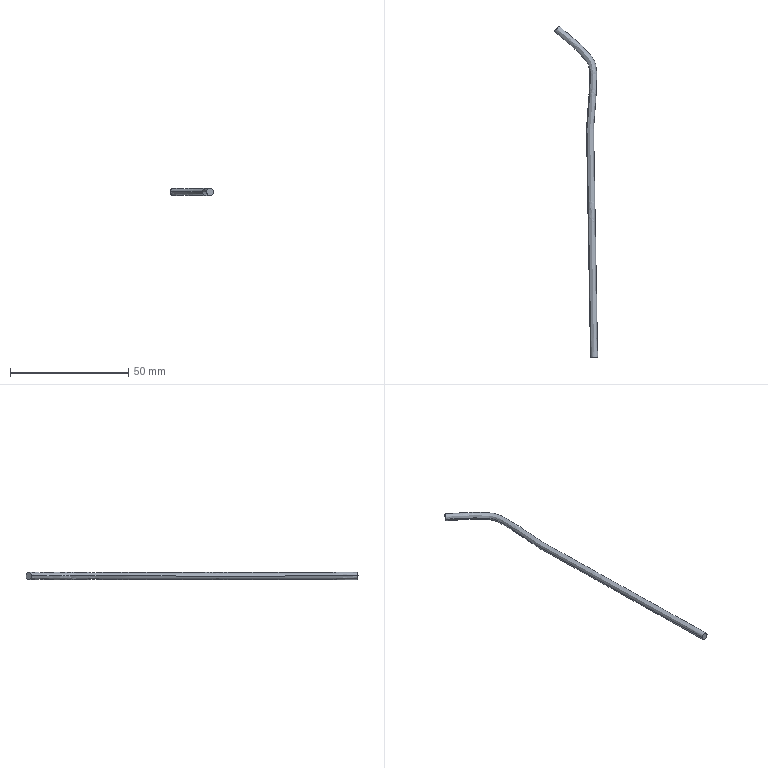Part | NX | features BREP 1 | 1 solid | 4 faces | box 18.288 x 140.353 x 3 mm | volume 1051 mm3 | spline 2 | plane 2
STEP:
#1=CARTESIAN_POINT('',(-100.98,103.131,217.465));
#2=VERTEX_POINT('',#1);
#3=CARTESIAN_POINT('',(-85.692,-34.901,217.465));
#4=VERTEX_POINT('',#3);
#5=CARTESIAN_POINT('',(-100.98,103.131,217.465));
#6=CARTESIAN_POINT('',(-99.807,102.169,217.465));
#7=CARTESIAN_POINT('',(-97.214,99.981,217.465));
#8=CARTESIAN_POINT('',(-94.267,97.623,217.465));
#9=CARTESIAN_POINT('',(-92.101,95.645,217.465));
#10=CARTESIAN_POINT('',(-90.487,94.026,217.465));
#11=CARTESIAN_POINT('',(-88.998,92.409,217.465));
#12=CARTESIAN_POINT('',(-87.788,91.003,217.465));
#13=CARTESIAN_POINT('',(-87.,89.888,217.465));
#14=CARTESIAN_POINT('',(-86.625,89.137,217.465));
#15=CARTESIAN_POINT('',(-86.388,88.253,217.465));
#16=CARTESIAN_POINT('',(-86.169,86.869,217.465));
#17=CARTESIAN_POINT('',(-86.049,85.054,217.465));
#18=CARTESIAN_POINT('',(-86.029,82.028,217.465));
#19=CARTESIAN_POINT('',(-86.155,79.005,217.465));
#20=CARTESIAN_POINT('',(-86.326,75.953,217.465));
#21=CARTESIAN_POINT('',(-86.474,73.619,217.465));
#22=CARTESIAN_POINT('',(-86.631,71.319,217.465));
#23=CARTESIAN_POINT('',(-86.81,68.899,217.465));
#24=CARTESIAN_POINT('',(-86.945,67.173,217.465));
#25=CARTESIAN_POINT('',(-87.031,66.14,217.465));
#26=CARTESIAN_POINT('',(-87.134,64.942,217.465));
#27=CARTESIAN_POINT('',(-87.22,64.02,217.465));
#28=CARTESIAN_POINT('',(-87.286,63.361,217.465));
#29=CARTESIAN_POINT('',(-87.349,62.799,217.465));
#30=CARTESIAN_POINT('',(-87.386,62.482,217.465));
#31=CARTESIAN_POINT('',(-87.402,62.06,217.465));
#32=CARTESIAN_POINT('',(-87.396,61.667,217.465));
#33=CARTESIAN_POINT('',(-87.394,60.965,217.465));
#34=CARTESIAN_POINT('',(-87.378,60.032,217.465));
#35=CARTESIAN_POINT('',(-87.364,59.116,217.465));
#36=CARTESIAN_POINT('',(-87.348,58.167,217.465));
#37=CARTESIAN_POINT('',(-87.32,56.62,217.465));
#38=CARTESIAN_POINT('',(-87.282,54.656,217.465));
#39=CARTESIAN_POINT('',(-87.217,51.348,217.465));
#40=CARTESIAN_POINT('',(-87.126,46.74,217.465));
#41=CARTESIAN_POINT('',(-87.017,40.936,217.465));
#42=CARTESIAN_POINT('',(-86.92,35.555,217.465));
#43=CARTESIAN_POINT('',(-86.84,30.908,217.465));
#44=CARTESIAN_POINT('',(-86.763,26.246,217.465));
#45=CARTESIAN_POINT('',(-86.69,21.778,217.465));
#46=CARTESIAN_POINT('',(-86.596,16.098,217.465));
#47=CARTESIAN_POINT('',(-86.483,9.497,217.465));
#48=CARTESIAN_POINT('',(-86.341,1.685,217.465));
#49=CARTESIAN_POINT('',(-86.183,-6.819,217.465));
#50=CARTESIAN_POINT('',(-86.012,-16.197,217.465));
#51=CARTESIAN_POINT('',(-85.857,-25.541,217.465));
#52=CARTESIAN_POINT('',(-85.752,-31.781,217.465));
#53=CARTESIAN_POINT('',(-85.692,-34.901,217.465));
#54=B_SPLINE_CURVE_WITH_KNOTS('',3,(#5,#6,#7,#8,#9,#10,#11,#12,#13,#14,#15,#16,#17,#18,#19,#20,#21,#22,#23,#24,#25,#26,#27,#28,#29,#30,#31,#32,#33,#34,#35,#36,#37,#38,#39,#40,#41,#42,#43,#44,#45,#46,#47,#48,#49,#50,#51,#52,#53),.UNSPECIFIED.,.F.,.F.,(4,1,1,1,1,1,1,1,1,1,1,1,1,1,1,1,1,1,1,1,1,1,1,1,1,1,1,1,1,1,1,1,1,1,1,1,1,1,1,1,1,1,1,1,1,1,4),(0.,0.03125,0.0625,0.07812,0.09375,0.1094,0.125,0.1328,0.1406,0.1484,0.1562,0.1719,0.1875,0.2188,0.2344,0.25,0.2656,0.2812,0.2969,0.3125,0.3203,0.3281,0.332,0.334,0.3359,0.3379,0.3398,0.3438,0.3516,0.3594,0.3672,0.375,0.3906,0.4062,0.4375,0.4688,0.5,0.5312,0.5625,0.5938,0.625,0.6875,0.75,0.8125,0.875,0.9375,1.),.UNSPECIFIED.);
#55=EDGE_CURVE('',#2,#4,#54,.T.);
#56=ORIENTED_EDGE('',*,*,#55,.T.);
#57=CARTESIAN_POINT('',(-82.692,-34.843,217.465));
#58=VERTEX_POINT('',#57);
#59=CARTESIAN_POINT('',(-85.692,-34.901,217.465));
#60=CARTESIAN_POINT('',(-85.692,-34.901,217.819));
#61=CARTESIAN_POINT('',(-85.424,-34.896,218.592));
#62=CARTESIAN_POINT('',(-84.192,-34.872,219.152));
#63=CARTESIAN_POINT('',(-82.96,-34.848,218.592));
#64=CARTESIAN_POINT('',(-82.692,-34.843,217.819));
#65=CARTESIAN_POINT('',(-82.692,-34.843,217.465));
#66=B_SPLINE_CURVE_WITH_KNOTS('',3,(#59,#60,#61,#62,#63,#64,#65),.UNSPECIFIED.,.F.,.F.,(4,1,1,1,4),(0.,0.25,0.5,0.75,1.),.UNSPECIFIED.);
#67=EDGE_CURVE('',#4,#58,#66,.T.);
#68=ORIENTED_EDGE('',*,*,#67,.T.);
#69=CARTESIAN_POINT('',(-99.08,105.451,217.465));
#70=VERTEX_POINT('',#69);
#71=CARTESIAN_POINT('',(-99.08,105.451,217.465));
#72=CARTESIAN_POINT('',(-98.296,104.81,217.465));
#73=CARTESIAN_POINT('',(-97.144,103.829,217.465));
#74=CARTESIAN_POINT('',(-95.558,102.527,217.465));
#75=CARTESIAN_POINT('',(-93.741,101.053,217.465));
#76=CARTESIAN_POINT('',(-91.797,99.446,217.465));
#77=CARTESIAN_POINT('',(-89.819,97.607,217.465));
#78=CARTESIAN_POINT('',(-88.587,96.367,217.465));
#79=CARTESIAN_POINT('',(-87.616,95.336,217.465));
#80=CARTESIAN_POINT('',(-86.681,94.308,217.465));
#81=CARTESIAN_POINT('',(-85.739,93.227,217.465));
#82=CARTESIAN_POINT('',(-84.766,91.955,217.465));
#83=CARTESIAN_POINT('',(-84.081,90.835,217.465));
#84=CARTESIAN_POINT('',(-83.601,89.552,217.465));
#85=CARTESIAN_POINT('',(-83.287,87.999,217.465));
#86=CARTESIAN_POINT('',(-83.109,86.257,217.465));
#87=CARTESIAN_POINT('',(-83.029,84.039,217.465));
#88=CARTESIAN_POINT('',(-83.054,81.652,217.465));
#89=CARTESIAN_POINT('',(-83.148,79.164,217.465));
#90=CARTESIAN_POINT('',(-83.278,76.688,217.465));
#91=CARTESIAN_POINT('',(-83.424,74.29,217.465));
#92=CARTESIAN_POINT('',(-83.553,72.364,217.465));
#93=CARTESIAN_POINT('',(-83.654,70.919,217.465));
#94=CARTESIAN_POINT('',(-83.758,69.487,217.465));
#95=CARTESIAN_POINT('',(-83.886,67.792,217.465));
#96=CARTESIAN_POINT('',(-83.988,66.538,217.465));
#97=CARTESIAN_POINT('',(-84.093,65.275,217.465));
#98=CARTESIAN_POINT('',(-84.215,63.901,217.465));
#99=CARTESIAN_POINT('',(-84.305,63.036,217.465));
#100=CARTESIAN_POINT('',(-84.335,62.759,217.465));
#101=CARTESIAN_POINT('',(-84.367,62.478,217.465));
#102=CARTESIAN_POINT('',(-84.392,62.258,217.465));
#103=CARTESIAN_POINT('',(-84.398,62.15,217.465));
#104=CARTESIAN_POINT('',(-84.399,61.903,217.465));
#105=CARTESIAN_POINT('',(-84.398,61.625,217.465));
#106=CARTESIAN_POINT('',(-84.393,61.053,217.465));
#107=CARTESIAN_POINT('',(-84.381,60.189,217.465));
#108=CARTESIAN_POINT('',(-84.366,59.251,217.465));
#109=CARTESIAN_POINT('',(-84.35,58.317,217.465));
#110=CARTESIAN_POINT('',(-84.302,55.696,217.465));
#111=CARTESIAN_POINT('',(-84.217,51.413,217.465));
#112=CARTESIAN_POINT('',(-84.083,44.513,217.465));
#113=CARTESIAN_POINT('',(-83.977,38.77,217.465));
#114=CARTESIAN_POINT('',(-83.905,34.702,217.465));
#115=CARTESIAN_POINT('',(-83.836,30.691,217.465));
#116=CARTESIAN_POINT('',(-83.751,25.529,217.465));
#117=CARTESIAN_POINT('',(-83.653,19.545,217.465));
#118=CARTESIAN_POINT('',(-83.559,13.961,217.465));
#119=CARTESIAN_POINT('',(-83.466,8.624,217.465));
#120=CARTESIAN_POINT('',(-83.37,3.287,217.465));
#121=CARTESIAN_POINT('',(-83.267,-2.297,217.465));
#122=CARTESIAN_POINT('',(-83.156,-8.279,217.465));
#123=CARTESIAN_POINT('',(-83.049,-14.191,217.465));
#124=CARTESIAN_POINT('',(-82.953,-19.683,217.465));
#125=CARTESIAN_POINT('',(-82.842,-26.423,217.465));
#126=CARTESIAN_POINT('',(-82.758,-31.476,217.465));
#127=CARTESIAN_POINT('',(-82.692,-34.843,217.465));
#128=B_SPLINE_CURVE_WITH_KNOTS('',3,(#71,#72,#73,#74,#75,#76,#77,#78,#79,#80,#81,#82,#83,#84,#85,#86,#87,#88,#89,#90,#91,#92,#93,#94,#95,#96,#97,#98,#99,#100,#101,#102,#103,#104,#105,#106,#107,#108,#109,#110,#111,#112,#113,#114,#115,#116,#117,#118,#119,#120,#121,#122,#123,#124,#125,#126,#127),.UNSPECIFIED.,.F.,.F.,(4,1,1,1,1,1,1,1,1,1,1,1,1,1,1,1,1,1,1,1,1,1,1,1,1,1,1,1,1,1,1,1,1,1,1,1,1,1,1,1,1,1,1,1,1,1,1,1,1,1,1,1,1,1,4),(0.,0.01978,0.02967,0.03956,0.06653,0.08001,0.09349,0.1006,0.1078,0.1221,0.1295,0.137,0.1442,0.1515,0.1647,0.1779,0.1947,0.2115,0.2282,0.245,0.2595,0.2668,0.274,0.288,0.302,0.3161,0.3301,0.3313,0.3326,0.3339,0.3352,0.3371,0.339,0.3409,0.3427,0.3507,0.3586,0.3665,0.3744,0.4121,0.4498,0.4874,0.5063,0.5251,0.5676,0.6101,0.6525,0.695,0.7375,0.7799,0.8224,0.8649,0.8987,0.9324,1.),.UNSPECIFIED.);
#129=EDGE_CURVE('',#70,#58,#128,.T.);
#130=ORIENTED_EDGE('',*,*,#129,.F.);
#131=CARTESIAN_POINT('',(-100.98,103.131,217.465));
#132=CARTESIAN_POINT('',(-100.98,103.131,217.819));
#133=CARTESIAN_POINT('',(-100.81,103.338,218.592));
#134=CARTESIAN_POINT('',(-100.03,104.291,219.152));
#135=CARTESIAN_POINT('',(-99.25,105.244,218.592));
#136=CARTESIAN_POINT('',(-99.08,105.451,217.819));
#137=CARTESIAN_POINT('',(-99.08,105.451,217.465));
#138=B_SPLINE_CURVE_WITH_KNOTS('',3,(#131,#132,#133,#134,#135,#136,#137),.UNSPECIFIED.,.F.,.F.,(4,1,1,1,4),(0.,0.25,0.5,0.75,1.),.UNSPECIFIED.);
#139=EDGE_CURVE('',#2,#70,#138,.T.);
#140=ORIENTED_EDGE('',*,*,#139,.F.);
#141=EDGE_LOOP('',(#56,#68,#130,#140));
#142=FACE_BOUND('',#141,.T.);
#143=CARTESIAN_POINT('',(-82.692,-34.843,217.465));
#144=CARTESIAN_POINT('',(-82.692,-34.843,217.819));
#145=CARTESIAN_POINT('',(-82.96,-34.848,218.592));
#146=CARTESIAN_POINT('',(-84.192,-34.872,219.152));
#147=CARTESIAN_POINT('',(-85.424,-34.896,218.592));
#148=CARTESIAN_POINT('',(-85.692,-34.901,217.819));
#149=CARTESIAN_POINT('',(-85.692,-34.901,217.465));
#150=CARTESIAN_POINT('',(-82.758,-31.476,217.465));
#151=CARTESIAN_POINT('',(-82.758,-31.476,217.819));
#152=CARTESIAN_POINT('',(-83.026,-31.481,218.592));
#153=CARTESIAN_POINT('',(-84.257,-31.502,219.152));
#154=CARTESIAN_POINT('',(-85.489,-31.524,218.592));
#155=CARTESIAN_POINT('',(-85.757,-31.529,217.819));
#156=CARTESIAN_POINT('',(-85.757,-31.529,217.465));
#157=CARTESIAN_POINT('',(-82.842,-26.423,217.465));
#158=CARTESIAN_POINT('',(-82.842,-26.423,217.819));
#159=CARTESIAN_POINT('',(-83.11,-26.427,218.592));
#160=CARTESIAN_POINT('',(-84.341,-26.447,219.152));
#161=CARTESIAN_POINT('',(-85.573,-26.467,218.592));
#162=CARTESIAN_POINT('',(-85.841,-26.472,217.819));
#163=CARTESIAN_POINT('',(-85.841,-26.472,217.465));
#164=CARTESIAN_POINT('',(-82.953,-19.683,217.465));
#165=CARTESIAN_POINT('',(-82.953,-19.683,217.819));
#166=CARTESIAN_POINT('',(-83.222,-19.687,218.592));
#167=CARTESIAN_POINT('',(-84.453,-19.708,219.152));
#168=CARTESIAN_POINT('',(-85.685,-19.729,218.592));
#169=CARTESIAN_POINT('',(-85.953,-19.734,217.819));
#170=CARTESIAN_POINT('',(-85.953,-19.734,217.465));
#171=CARTESIAN_POINT('',(-83.049,-14.191,217.465));
#172=CARTESIAN_POINT('',(-83.049,-14.191,217.819));
#173=CARTESIAN_POINT('',(-83.317,-14.195,218.592));
#174=CARTESIAN_POINT('',(-84.549,-14.217,219.152));
#175=CARTESIAN_POINT('',(-85.78,-14.239,218.592));
#176=CARTESIAN_POINT('',(-86.048,-14.244,217.819));
#177=CARTESIAN_POINT('',(-86.048,-14.244,217.465));
#178=CARTESIAN_POINT('',(-83.156,-8.279,217.465));
#179=CARTESIAN_POINT('',(-83.156,-8.279,217.819));
#180=CARTESIAN_POINT('',(-83.424,-8.284,218.592));
#181=CARTESIAN_POINT('',(-84.656,-8.306,219.152));
#182=CARTESIAN_POINT('',(-85.887,-8.329,218.592));
#183=CARTESIAN_POINT('',(-86.155,-8.334,217.819));
#184=CARTESIAN_POINT('',(-86.155,-8.334,217.465));
#185=CARTESIAN_POINT('',(-83.267,-2.297,217.465));
#186=CARTESIAN_POINT('',(-83.267,-2.297,217.819));
#187=CARTESIAN_POINT('',(-83.535,-2.302,218.592));
#188=CARTESIAN_POINT('',(-84.766,-2.325,219.152));
#189=CARTESIAN_POINT('',(-85.998,-2.348,218.592));
#190=CARTESIAN_POINT('',(-86.266,-2.353,217.819));
#191=CARTESIAN_POINT('',(-86.266,-2.353,217.465));
#192=CARTESIAN_POINT('',(-83.37,3.287,217.465));
#193=CARTESIAN_POINT('',(-83.37,3.287,217.819));
#194=CARTESIAN_POINT('',(-83.638,3.283,218.592));
#195=CARTESIAN_POINT('',(-84.87,3.26,219.152));
#196=CARTESIAN_POINT('',(-86.101,3.238,218.592));
#197=CARTESIAN_POINT('',(-86.369,3.233,217.819));
#198=CARTESIAN_POINT('',(-86.369,3.233,217.465));
#199=CARTESIAN_POINT('',(-83.466,8.624,217.465));
#200=CARTESIAN_POINT('',(-83.466,8.624,217.819));
#201=CARTESIAN_POINT('',(-83.735,8.62,218.592));
#202=CARTESIAN_POINT('',(-84.966,8.598,219.152));
#203=CARTESIAN_POINT('',(-86.198,8.577,218.592));
#204=CARTESIAN_POINT('',(-86.466,8.572,217.819));
#205=CARTESIAN_POINT('',(-86.466,8.572,217.465));
#206=CARTESIAN_POINT('',(-83.559,13.961,217.465));
#207=CARTESIAN_POINT('',(-83.559,13.961,217.819));
#208=CARTESIAN_POINT('',(-83.827,13.957,218.592));
#209=CARTESIAN_POINT('',(-85.059,13.936,219.152));
#210=CARTESIAN_POINT('',(-86.291,13.916,218.592));
#211=CARTESIAN_POINT('',(-86.559,13.911,217.819));
#212=CARTESIAN_POINT('',(-86.559,13.911,217.465));
#213=CARTESIAN_POINT('',(-83.653,19.545,217.465));
#214=CARTESIAN_POINT('',(-83.653,19.545,217.819));
#215=CARTESIAN_POINT('',(-83.921,19.541,218.592));
#216=CARTESIAN_POINT('',(-85.152,19.521,219.152));
#217=CARTESIAN_POINT('',(-86.384,19.501,218.592));
#218=CARTESIAN_POINT('',(-86.652,19.496,217.819));
#219=CARTESIAN_POINT('',(-86.652,19.496,217.465));
#220=CARTESIAN_POINT('',(-83.751,25.529,217.465));
#221=CARTESIAN_POINT('',(-83.751,25.529,217.819));
#222=CARTESIAN_POINT('',(-84.019,25.525,218.592));
#223=CARTESIAN_POINT('',(-85.25,25.505,219.152));
#224=CARTESIAN_POINT('',(-86.482,25.485,218.592));
#225=CARTESIAN_POINT('',(-86.75,25.48,217.819));
#226=CARTESIAN_POINT('',(-86.75,25.48,217.465));
#227=CARTESIAN_POINT('',(-83.836,30.691,217.465));
#228=CARTESIAN_POINT('',(-83.836,30.691,217.819));
#229=CARTESIAN_POINT('',(-84.104,30.687,218.592));
#230=CARTESIAN_POINT('',(-85.336,30.666,219.152));
#231=CARTESIAN_POINT('',(-86.567,30.645,218.592));
#232=CARTESIAN_POINT('',(-86.836,30.641,217.819));
#233=CARTESIAN_POINT('',(-86.836,30.641,217.465));
#234=CARTESIAN_POINT('',(-83.905,34.702,217.465));
#235=CARTESIAN_POINT('',(-83.905,34.702,217.819));
#236=CARTESIAN_POINT('',(-84.173,34.697,218.592));
#237=CARTESIAN_POINT('',(-85.404,34.676,219.152));
#238=CARTESIAN_POINT('',(-86.636,34.655,218.592));
#239=CARTESIAN_POINT('',(-86.904,34.65,217.819));
#240=CARTESIAN_POINT('',(-86.904,34.65,217.465));
#241=CARTESIAN_POINT('',(-83.977,38.77,217.465));
#242=CARTESIAN_POINT('',(-83.977,38.77,217.819));
#243=CARTESIAN_POINT('',(-84.245,38.765,218.592));
#244=CARTESIAN_POINT('',(-85.476,38.743,219.152));
#245=CARTESIAN_POINT('',(-86.708,38.721,218.592));
#246=CARTESIAN_POINT('',(-86.976,38.716,217.819));
#247=CARTESIAN_POINT('',(-86.976,38.716,217.465));
#248=CARTESIAN_POINT('',(-84.083,44.513,217.465));
#249=CARTESIAN_POINT('',(-84.083,44.513,217.819));
#250=CARTESIAN_POINT('',(-84.351,44.508,218.592));
#251=CARTESIAN_POINT('',(-85.582,44.485,219.152));
#252=CARTESIAN_POINT('',(-86.814,44.463,218.592));
#253=CARTESIAN_POINT('',(-87.082,44.458,217.819));
#254=CARTESIAN_POINT('',(-87.082,44.458,217.465));
#255=CARTESIAN_POINT('',(-84.217,51.413,217.465));
#256=CARTESIAN_POINT('',(-84.217,51.413,217.819));
#257=CARTESIAN_POINT('',(-84.485,51.407,218.592));
#258=CARTESIAN_POINT('',(-85.717,51.384,219.152));
#259=CARTESIAN_POINT('',(-86.948,51.36,218.592));
#260=CARTESIAN_POINT('',(-87.216,51.355,217.819));
#261=CARTESIAN_POINT('',(-87.216,51.355,217.465));
#262=CARTESIAN_POINT('',(-84.302,55.696,217.465));
#263=CARTESIAN_POINT('',(-84.302,55.696,217.819));
#264=CARTESIAN_POINT('',(-84.57,55.691,218.592));
#265=CARTESIAN_POINT('',(-85.802,55.666,219.152));
#266=CARTESIAN_POINT('',(-87.033,55.642,218.592));
#267=CARTESIAN_POINT('',(-87.302,55.636,217.819));
#268=CARTESIAN_POINT('',(-87.302,55.636,217.465));
#269=CARTESIAN_POINT('',(-84.35,58.317,217.465));
#270=CARTESIAN_POINT('',(-84.35,58.317,217.819));
#271=CARTESIAN_POINT('',(-84.618,58.312,218.592));
#272=CARTESIAN_POINT('',(-85.85,58.29,219.152));
#273=CARTESIAN_POINT('',(-87.081,58.269,218.592));
#274=CARTESIAN_POINT('',(-87.349,58.264,217.819));
#275=CARTESIAN_POINT('',(-87.349,58.264,217.465));
#276=CARTESIAN_POINT('',(-84.366,59.251,217.465));
#277=CARTESIAN_POINT('',(-84.366,59.251,217.819));
#278=CARTESIAN_POINT('',(-84.634,59.247,218.592));
#279=CARTESIAN_POINT('',(-85.866,59.229,219.152));
#280=CARTESIAN_POINT('',(-87.097,59.21,218.592));
#281=CARTESIAN_POINT('',(-87.365,59.206,217.819));
#282=CARTESIAN_POINT('',(-87.365,59.206,217.465));
#283=CARTESIAN_POINT('',(-84.381,60.189,217.465));
#284=CARTESIAN_POINT('',(-84.381,60.189,217.819));
#285=CARTESIAN_POINT('',(-84.649,60.186,218.592));
#286=CARTESIAN_POINT('',(-85.881,60.169,219.152));
#287=CARTESIAN_POINT('',(-87.113,60.152,218.592));
#288=CARTESIAN_POINT('',(-87.381,60.149,217.819));
#289=CARTESIAN_POINT('',(-87.381,60.149,217.465));
#290=CARTESIAN_POINT('',(-84.393,61.053,217.465));
#291=CARTESIAN_POINT('',(-84.393,61.053,217.819));
#292=CARTESIAN_POINT('',(-84.661,61.05,218.592));
#293=CARTESIAN_POINT('',(-85.893,61.033,219.152));
#294=CARTESIAN_POINT('',(-87.125,61.017,218.592));
#295=CARTESIAN_POINT('',(-87.393,61.013,217.819));
#296=CARTESIAN_POINT('',(-87.393,61.013,217.465));
#297=CARTESIAN_POINT('',(-84.398,61.625,217.465));
#298=CARTESIAN_POINT('',(-84.398,61.625,217.819));
#299=CARTESIAN_POINT('',(-84.666,61.623,218.592));
#300=CARTESIAN_POINT('',(-85.898,61.616,219.152));
#301=CARTESIAN_POINT('',(-87.13,61.609,218.592));
#302=CARTESIAN_POINT('',(-87.398,61.608,217.819));
#303=CARTESIAN_POINT('',(-87.398,61.608,217.465));
#304=CARTESIAN_POINT('',(-84.399,61.903,217.465));
#305=CARTESIAN_POINT('',(-84.399,61.903,217.819));
#306=CARTESIAN_POINT('',(-84.667,61.902,218.592));
#307=CARTESIAN_POINT('',(-85.898,61.899,219.152));
#308=CARTESIAN_POINT('',(-87.13,61.895,218.592));
#309=CARTESIAN_POINT('',(-87.398,61.895,217.819));
#310=CARTESIAN_POINT('',(-87.398,61.895,217.465));
#311=CARTESIAN_POINT('',(-84.398,62.15,217.465));
#312=CARTESIAN_POINT('',(-84.398,62.15,217.819));
#313=CARTESIAN_POINT('',(-84.667,62.156,218.592));
#314=CARTESIAN_POINT('',(-85.9,62.182,219.152));
#315=CARTESIAN_POINT('',(-87.132,62.207,218.592));
#316=CARTESIAN_POINT('',(-87.401,62.213,217.819));
#317=CARTESIAN_POINT('',(-87.401,62.213,217.465));
#318=CARTESIAN_POINT('',(-84.392,62.258,217.465));
#319=CARTESIAN_POINT('',(-84.392,62.258,217.819));
#320=CARTESIAN_POINT('',(-84.659,62.288,218.592));
#321=CARTESIAN_POINT('',(-85.884,62.425,219.152));
#322=CARTESIAN_POINT('',(-87.108,62.562,218.592));
#323=CARTESIAN_POINT('',(-87.375,62.592,217.819));
#324=CARTESIAN_POINT('',(-87.375,62.592,217.465));
#325=CARTESIAN_POINT('',(-84.367,62.478,217.465));
#326=CARTESIAN_POINT('',(-84.367,62.478,217.819));
#327=CARTESIAN_POINT('',(-84.633,62.509,218.592));
#328=CARTESIAN_POINT('',(-85.857,62.65,219.152));
#329=CARTESIAN_POINT('',(-87.08,62.79,218.592));
#330=CARTESIAN_POINT('',(-87.347,62.821,217.819));
#331=CARTESIAN_POINT('',(-87.347,62.821,217.465));
#332=CARTESIAN_POINT('',(-84.335,62.759,217.465));
#333=CARTESIAN_POINT('',(-84.335,62.759,217.819));
#334=CARTESIAN_POINT('',(-84.602,62.788,218.592));
#335=CARTESIAN_POINT('',(-85.826,62.92,219.152));
#336=CARTESIAN_POINT('',(-87.051,63.053,218.592));
#337=CARTESIAN_POINT('',(-87.317,63.081,217.819));
#338=CARTESIAN_POINT('',(-87.317,63.081,217.465));
#339=CARTESIAN_POINT('',(-84.305,63.036,217.465));
#340=CARTESIAN_POINT('',(-84.305,63.036,217.819));
#341=CARTESIAN_POINT('',(-84.572,63.065,218.592));
#342=CARTESIAN_POINT('',(-85.797,63.193,219.152));
#343=CARTESIAN_POINT('',(-87.022,63.322,218.592));
#344=CARTESIAN_POINT('',(-87.289,63.35,217.819));
#345=CARTESIAN_POINT('',(-87.289,63.35,217.465));
#346=CARTESIAN_POINT('',(-84.215,63.901,217.465));
#347=CARTESIAN_POINT('',(-84.215,63.901,217.819));
#348=CARTESIAN_POINT('',(-84.482,63.926,218.592));
#349=CARTESIAN_POINT('',(-85.709,64.041,219.152));
#350=CARTESIAN_POINT('',(-86.935,64.157,218.592));
#351=CARTESIAN_POINT('',(-87.202,64.182,217.819));
#352=CARTESIAN_POINT('',(-87.202,64.182,217.465));
#353=CARTESIAN_POINT('',(-84.093,65.275,217.465));
#354=CARTESIAN_POINT('',(-84.093,65.275,217.819));
#355=CARTESIAN_POINT('',(-84.361,65.299,218.592));
#356=CARTESIAN_POINT('',(-85.587,65.407,219.152));
#357=CARTESIAN_POINT('',(-86.814,65.515,218.592));
#358=CARTESIAN_POINT('',(-87.081,65.539,217.819));
#359=CARTESIAN_POINT('',(-87.081,65.539,217.465));
#360=CARTESIAN_POINT('',(-83.988,66.538,217.465));
#361=CARTESIAN_POINT('',(-83.988,66.538,217.819));
#362=CARTESIAN_POINT('',(-84.255,66.561,218.592));
#363=CARTESIAN_POINT('',(-85.482,66.667,219.152));
#364=CARTESIAN_POINT('',(-86.709,66.772,218.592));
#365=CARTESIAN_POINT('',(-86.976,66.795,217.819));
#366=CARTESIAN_POINT('',(-86.976,66.795,217.465));
#367=CARTESIAN_POINT('',(-83.886,67.792,217.465));
#368=CARTESIAN_POINT('',(-83.886,67.792,217.819));
#369=CARTESIAN_POINT('',(-84.154,67.813,218.592));
#370=CARTESIAN_POINT('',(-85.382,67.909,219.152));
#371=CARTESIAN_POINT('',(-86.61,68.006,218.592));
#372=CARTESIAN_POINT('',(-86.877,68.027,217.819));
#373=CARTESIAN_POINT('',(-86.877,68.027,217.465));
#374=CARTESIAN_POINT('',(-83.758,69.487,217.465));
#375=CARTESIAN_POINT('',(-83.758,69.487,217.819));
#376=CARTESIAN_POINT('',(-84.025,69.507,218.592));
#377=CARTESIAN_POINT('',(-85.254,69.598,219.152));
#378=CARTESIAN_POINT('',(-86.482,69.689,218.592));
#379=CARTESIAN_POINT('',(-86.749,69.709,217.819));
#380=CARTESIAN_POINT('',(-86.749,69.709,217.465));
#381=CARTESIAN_POINT('',(-83.654,70.919,217.465));
#382=CARTESIAN_POINT('',(-83.654,70.919,217.819));
#383=CARTESIAN_POINT('',(-83.922,70.938,218.592));
#384=CARTESIAN_POINT('',(-85.15,71.026,219.152));
#385=CARTESIAN_POINT('',(-86.379,71.113,218.592));
#386=CARTESIAN_POINT('',(-86.646,71.133,217.819));
#387=CARTESIAN_POINT('',(-86.646,71.133,217.465));
#388=CARTESIAN_POINT('',(-83.553,72.364,217.465));
#389=CARTESIAN_POINT('',(-83.553,72.364,217.819));
#390=CARTESIAN_POINT('',(-83.82,72.383,218.592));
#391=CARTESIAN_POINT('',(-85.049,72.466,219.152));
#392=CARTESIAN_POINT('',(-86.278,72.55,218.592));
#393=CARTESIAN_POINT('',(-86.546,72.569,217.819));
#394=CARTESIAN_POINT('',(-86.546,72.569,217.465));
#395=CARTESIAN_POINT('',(-83.424,74.29,217.465));
#396=CARTESIAN_POINT('',(-83.424,74.29,217.819));
#397=CARTESIAN_POINT('',(-83.692,74.307,218.592));
#398=CARTESIAN_POINT('',(-84.921,74.386,219.152));
#399=CARTESIAN_POINT('',(-86.15,74.465,218.592));
#400=CARTESIAN_POINT('',(-86.418,74.482,217.819));
#401=CARTESIAN_POINT('',(-86.418,74.482,217.465));
#402=CARTESIAN_POINT('',(-83.278,76.688,217.465));
#403=CARTESIAN_POINT('',(-83.278,76.688,217.819));
#404=CARTESIAN_POINT('',(-83.546,76.703,218.592));
#405=CARTESIAN_POINT('',(-84.775,76.774,219.152));
#406=CARTESIAN_POINT('',(-86.005,76.844,218.592));
#407=CARTESIAN_POINT('',(-86.273,76.86,217.819));
#408=CARTESIAN_POINT('',(-86.273,76.86,217.465));
#409=CARTESIAN_POINT('',(-83.148,79.164,217.465));
#410=CARTESIAN_POINT('',(-83.148,79.164,217.819));
#411=CARTESIAN_POINT('',(-83.416,79.177,218.592));
#412=CARTESIAN_POINT('',(-84.646,79.234,219.152));
#413=CARTESIAN_POINT('',(-85.877,79.291,218.592));
#414=CARTESIAN_POINT('',(-86.145,79.303,217.819));
#415=CARTESIAN_POINT('',(-86.145,79.303,217.465));
#416=CARTESIAN_POINT('',(-83.054,81.652,217.465));
#417=CARTESIAN_POINT('',(-83.054,81.652,217.819));
#418=CARTESIAN_POINT('',(-83.322,81.659,218.592));
#419=CARTESIAN_POINT('',(-84.554,81.692,219.152));
#420=CARTESIAN_POINT('',(-85.785,81.725,218.592));
#421=CARTESIAN_POINT('',(-86.053,81.732,217.819));
#422=CARTESIAN_POINT('',(-86.053,81.732,217.465));
#423=CARTESIAN_POINT('',(-83.029,84.039,217.465));
#424=CARTESIAN_POINT('',(-83.029,84.039,217.819));
#425=CARTESIAN_POINT('',(-83.297,84.038,218.592));
#426=CARTESIAN_POINT('',(-84.529,84.029,219.152));
#427=CARTESIAN_POINT('',(-85.762,84.021,218.592));
#428=CARTESIAN_POINT('',(-86.03,84.019,217.819));
#429=CARTESIAN_POINT('',(-86.03,84.019,217.465));
#430=CARTESIAN_POINT('',(-83.109,86.257,217.465));
#431=CARTESIAN_POINT('',(-83.109,86.257,217.819));
#432=CARTESIAN_POINT('',(-83.377,86.24,218.592));
#433=CARTESIAN_POINT('',(-84.606,86.159,219.152));
#434=CARTESIAN_POINT('',(-85.836,86.078,218.592));
#435=CARTESIAN_POINT('',(-86.103,86.06,217.819));
#436=CARTESIAN_POINT('',(-86.103,86.06,217.465));
#437=CARTESIAN_POINT('',(-83.287,87.999,217.465));
#438=CARTESIAN_POINT('',(-83.287,87.999,217.819));
#439=CARTESIAN_POINT('',(-83.553,87.963,218.592));
#440=CARTESIAN_POINT('',(-84.775,87.8,219.152));
#441=CARTESIAN_POINT('',(-85.998,87.636,218.592));
#442=CARTESIAN_POINT('',(-86.264,87.601,217.819));
#443=CARTESIAN_POINT('',(-86.264,87.601,217.465));
#444=CARTESIAN_POINT('',(-83.601,89.552,217.465));
#445=CARTESIAN_POINT('',(-83.601,89.552,217.819));
#446=CARTESIAN_POINT('',(-83.861,89.481,218.592));
#447=CARTESIAN_POINT('',(-85.055,89.156,219.152));
#448=CARTESIAN_POINT('',(-86.249,88.831,218.592));
#449=CARTESIAN_POINT('',(-86.509,88.76,217.819));
#450=CARTESIAN_POINT('',(-86.509,88.76,217.465));
#451=CARTESIAN_POINT('',(-84.081,90.835,217.465));
#452=CARTESIAN_POINT('',(-84.081,90.835,217.819));
#453=CARTESIAN_POINT('',(-84.322,90.715,218.592));
#454=CARTESIAN_POINT('',(-85.431,90.161,219.152));
#455=CARTESIAN_POINT('',(-86.54,89.608,218.592));
#456=CARTESIAN_POINT('',(-86.781,89.488,217.819));
#457=CARTESIAN_POINT('',(-86.781,89.488,217.465));
#458=CARTESIAN_POINT('',(-84.766,91.955,217.465));
#459=CARTESIAN_POINT('',(-84.766,91.955,217.819));
#460=CARTESIAN_POINT('',(-84.986,91.801,218.592));
#461=CARTESIAN_POINT('',(-85.996,91.091,219.152));
#462=CARTESIAN_POINT('',(-87.006,90.382,218.592));
#463=CARTESIAN_POINT('',(-87.225,90.228,217.819));
#464=CARTESIAN_POINT('',(-87.225,90.228,217.465));
#465=CARTESIAN_POINT('',(-85.739,93.227,217.465));
#466=CARTESIAN_POINT('',(-85.739,93.227,217.819));
#467=CARTESIAN_POINT('',(-85.944,93.054,218.592));
#468=CARTESIAN_POINT('',(-86.886,92.259,219.152));
#469=CARTESIAN_POINT('',(-87.828,91.465,218.592));
#470=CARTESIAN_POINT('',(-88.033,91.292,217.819));
#471=CARTESIAN_POINT('',(-88.033,91.292,217.465));
#472=CARTESIAN_POINT('',(-86.681,94.308,217.465));
#473=CARTESIAN_POINT('',(-86.681,94.308,217.819));
#474=CARTESIAN_POINT('',(-86.882,94.13,218.592));
#475=CARTESIAN_POINT('',(-87.805,93.314,219.152));
#476=CARTESIAN_POINT('',(-88.727,92.498,218.592));
#477=CARTESIAN_POINT('',(-88.928,92.321,217.819));
#478=CARTESIAN_POINT('',(-88.928,92.321,217.465));
#479=CARTESIAN_POINT('',(-87.616,95.336,217.465));
#480=CARTESIAN_POINT('',(-87.616,95.336,217.819));
#481=CARTESIAN_POINT('',(-87.813,95.153,218.592));
#482=CARTESIAN_POINT('',(-88.717,94.317,219.152));
#483=CARTESIAN_POINT('',(-89.621,93.48,218.592));
#484=CARTESIAN_POINT('',(-89.817,93.298,217.819));
#485=CARTESIAN_POINT('',(-89.817,93.298,217.465));
#486=CARTESIAN_POINT('',(-88.587,96.367,217.465));
#487=CARTESIAN_POINT('',(-88.587,96.367,217.819));
#488=CARTESIAN_POINT('',(-88.779,96.18,218.592));
#489=CARTESIAN_POINT('',(-89.664,95.323,219.152));
#490=CARTESIAN_POINT('',(-90.549,94.466,218.592));
#491=CARTESIAN_POINT('',(-90.742,94.279,217.819));
#492=CARTESIAN_POINT('',(-90.742,94.279,217.465));
#493=CARTESIAN_POINT('',(-89.819,97.607,217.465));
#494=CARTESIAN_POINT('',(-89.819,97.607,217.819));
#495=CARTESIAN_POINT('',(-90.006,97.414,218.592));
#496=CARTESIAN_POINT('',(-90.863,96.529,219.152));
#497=CARTESIAN_POINT('',(-91.72,95.644,218.592));
#498=CARTESIAN_POINT('',(-91.907,95.451,217.819));
#499=CARTESIAN_POINT('',(-91.907,95.451,217.465));
#500=CARTESIAN_POINT('',(-91.797,99.446,217.465));
#501=CARTESIAN_POINT('',(-91.797,99.446,217.819));
#502=CARTESIAN_POINT('',(-91.972,99.243,218.592));
#503=CARTESIAN_POINT('',(-92.78,98.313,219.152));
#504=CARTESIAN_POINT('',(-93.588,97.382,218.592));
#505=CARTESIAN_POINT('',(-93.764,97.179,217.819));
#506=CARTESIAN_POINT('',(-93.764,97.179,217.465));
#507=CARTESIAN_POINT('',(-93.741,101.053,217.465));
#508=CARTESIAN_POINT('',(-93.741,101.053,217.819));
#509=CARTESIAN_POINT('',(-93.91,100.845,218.592));
#510=CARTESIAN_POINT('',(-94.685,99.888,219.152));
#511=CARTESIAN_POINT('',(-95.46,98.93,218.592));
#512=CARTESIAN_POINT('',(-95.629,98.722,217.819));
#513=CARTESIAN_POINT('',(-95.629,98.722,217.465));
#514=CARTESIAN_POINT('',(-95.558,102.527,217.465));
#515=CARTESIAN_POINT('',(-95.558,102.527,217.819));
#516=CARTESIAN_POINT('',(-95.727,102.319,218.592));
#517=CARTESIAN_POINT('',(-96.505,101.364,219.152));
#518=CARTESIAN_POINT('',(-97.283,100.409,218.592));
#519=CARTESIAN_POINT('',(-97.452,100.201,217.819));
#520=CARTESIAN_POINT('',(-97.452,100.201,217.465));
#521=CARTESIAN_POINT('',(-97.144,103.829,217.465));
#522=CARTESIAN_POINT('',(-97.144,103.829,217.819));
#523=CARTESIAN_POINT('',(-97.316,103.623,218.592));
#524=CARTESIAN_POINT('',(-98.104,102.677,219.152));
#525=CARTESIAN_POINT('',(-98.892,101.73,218.592));
#526=CARTESIAN_POINT('',(-99.064,101.524,217.819));
#527=CARTESIAN_POINT('',(-99.064,101.524,217.465));
#528=CARTESIAN_POINT('',(-98.296,104.81,217.465));
#529=CARTESIAN_POINT('',(-98.296,104.81,217.819));
#530=CARTESIAN_POINT('',(-98.47,104.605,218.592));
#531=CARTESIAN_POINT('',(-99.267,103.666,219.152));
#532=CARTESIAN_POINT('',(-100.064,102.726,218.592));
#533=CARTESIAN_POINT('',(-100.237,102.522,217.819));
#534=CARTESIAN_POINT('',(-100.237,102.522,217.465));
#535=CARTESIAN_POINT('',(-99.08,105.451,217.465));
#536=CARTESIAN_POINT('',(-99.08,105.451,217.819));
#537=CARTESIAN_POINT('',(-99.25,105.244,218.592));
#538=CARTESIAN_POINT('',(-100.03,104.291,219.152));
#539=CARTESIAN_POINT('',(-100.81,103.338,218.592));
#540=CARTESIAN_POINT('',(-100.98,103.131,217.819));
#541=CARTESIAN_POINT('',(-100.98,103.131,217.465));
#542=B_SPLINE_SURFACE_WITH_KNOTS('',3,3,((#143,#144,#145,#146,#147,#148,#149),(#150,#151,#152,#153,#154,#155,#156),(#157,#158,#159,#160,#161,#162,#163),(#164,#165,#166,#167,#168,#169,#170),(#171,#172,#173,#174,#175,#176,#177),(#178,#179,#180,#181,#182,#183,#184),(#185,#186,#187,#188,#189,#190,#191),(#192,#193,#194,#195,#196,#197,#198),(#199,#200,#201,#202,#203,#204,#205),(#206,#207,#208,#209,#210,#211,#212),(#213,#214,#215,#216,#217,#218,#219),(#220,#221,#222,#223,#224,#225,#226),(#227,#228,#229,#230,#231,#232,#233),(#234,#235,#236,#237,#238,#239,#240),(#241,#242,#243,#244,#245,#246,#247),(#248,#249,#250,#251,#252,#253,#254),(#255,#256,#257,#258,#259,#260,#261),(#262,#263,#264,#265,#266,#267,#268),(#269,#270,#271,#272,#273,#274,#275),(#276,#277,#278,#279,#280,#281,#282),(#283,#284,#285,#286,#287,#288,#289),(#290,#291,#292,#293,#294,#295,#296),(#297,#298,#299,#300,#301,#302,#303),(#304,#305,#306,#307,#308,#309,#310),(#311,#312,#313,#314,#315,#316,#317),(#318,#319,#320,#321,#322,#323,#324),(#325,#326,#327,#328,#329,#330,#331),(#332,#333,#334,#335,#336,#337,#338),(#339,#340,#341,#342,#343,#344,#345),(#346,#347,#348,#349,#350,#351,#352),(#353,#354,#355,#356,#357,#358,#359),(#360,#361,#362,#363,#364,#365,#366),(#367,#368,#369,#370,#371,#372,#373),(#374,#375,#376,#377,#378,#379,#380),(#381,#382,#383,#384,#385,#386,#387),(#388,#389,#390,#391,#392,#393,#394),(#395,#396,#397,#398,#399,#400,#401),(#402,#403,#404,#405,#406,#407,#408),(#409,#410,#411,#412,#413,#414,#415),(#416,#417,#418,#419,#420,#421,#422),(#423,#424,#425,#426,#427,#428,#429),(#430,#431,#432,#433,#434,#435,#436),(#437,#438,#439,#440,#441,#442,#443),(#444,#445,#446,#447,#448,#449,#450),(#451,#452,#453,#454,#455,#456,#457),(#458,#459,#460,#461,#462,#463,#464),(#465,#466,#467,#468,#469,#470,#471),(#472,#473,#474,#475,#476,#477,#478),(#479,#480,#481,#482,#483,#484,#485),(#486,#487,#488,#489,#490,#491,#492),(#493,#494,#495,#496,#497,#498,#499),(#500,#501,#502,#503,#504,#505,#506),(#507,#508,#509,#510,#511,#512,#513),(#514,#515,#516,#517,#518,#519,#520),(#521,#522,#523,#524,#525,#526,#527),(#528,#529,#530,#531,#532,#533,#534),(#535,#536,#537,#538,#539,#540,#541)),.UNSPECIFIED.,.F.,.F.,.F.,(4,1,1,1,1,1,1,1,1,1,1,1,1,1,1,1,1,1,1,1,1,1,1,1,1,1,1,1,1,1,1,1,1,1,1,1,1,1,1,1,1,1,1,1,1,1,1,1,1,1,1,1,1,1,4),(4,1,1,1,4),(0.009472,0.07575,0.1089,0.142,0.1837,0.2254,0.2671,0.3087,0.3504,0.3921,0.4337,0.4754,0.4939,0.5124,0.5494,0.5863,0.6233,0.6311,0.6388,0.6466,0.6544,0.6562,0.658,0.6599,0.6618,0.663,0.6643,0.6655,0.6668,0.6805,0.6943,0.708,0.7218,0.7289,0.736,0.7502,0.7667,0.7832,0.7996,0.8161,0.8291,0.842,0.8491,0.8562,0.8635,0.8708,0.8849,0.8919,0.8989,0.9121,0.9254,0.9518,0.9615,0.9712,0.9906),(0.02151,0.2608,0.5002,0.7395,0.9788),.UNSPECIFIED.);
#543=ADVANCED_FACE('',(#142),#542,.T.);
#544=ORIENTED_EDGE('',*,*,#129,.T.);
#545=CARTESIAN_POINT('',(-82.692,-34.843,217.465));
#546=CARTESIAN_POINT('',(-82.692,-34.843,217.111));
#547=CARTESIAN_POINT('',(-82.96,-34.848,216.338));
#548=CARTESIAN_POINT('',(-84.192,-34.872,215.778));
#549=CARTESIAN_POINT('',(-85.424,-34.896,216.338));
#550=CARTESIAN_POINT('',(-85.692,-34.901,217.111));
#551=CARTESIAN_POINT('',(-85.692,-34.901,217.465));
#552=B_SPLINE_CURVE_WITH_KNOTS('',3,(#545,#546,#547,#548,#549,#550,#551),.UNSPECIFIED.,.F.,.F.,(4,1,1,1,4),(0.,0.25,0.5,0.75,1.),.UNSPECIFIED.);
#553=EDGE_CURVE('',#58,#4,#552,.T.);
#554=ORIENTED_EDGE('',*,*,#553,.T.);
#555=ORIENTED_EDGE('',*,*,#55,.F.);
#556=CARTESIAN_POINT('',(-99.08,105.451,217.465));
#557=CARTESIAN_POINT('',(-99.08,105.451,217.111));
#558=CARTESIAN_POINT('',(-99.25,105.244,216.338));
#559=CARTESIAN_POINT('',(-100.03,104.291,215.778));
#560=CARTESIAN_POINT('',(-100.81,103.338,216.338));
#561=CARTESIAN_POINT('',(-100.98,103.131,217.111));
#562=CARTESIAN_POINT('',(-100.98,103.131,217.465));
#563=B_SPLINE_CURVE_WITH_KNOTS('',3,(#556,#557,#558,#559,#560,#561,#562),.UNSPECIFIED.,.F.,.F.,(4,1,1,1,4),(0.,0.25,0.5,0.75,1.),.UNSPECIFIED.);
#564=EDGE_CURVE('',#70,#2,#563,.T.);
#565=ORIENTED_EDGE('',*,*,#564,.F.);
#566=EDGE_LOOP('',(#544,#554,#555,#565));
#567=FACE_BOUND('',#566,.T.);
#568=CARTESIAN_POINT('',(-85.692,-34.901,217.465));
#569=CARTESIAN_POINT('',(-85.692,-34.901,217.111));
#570=CARTESIAN_POINT('',(-85.424,-34.896,216.338));
#571=CARTESIAN_POINT('',(-84.192,-34.872,215.778));
#572=CARTESIAN_POINT('',(-82.96,-34.848,216.338));
#573=CARTESIAN_POINT('',(-82.692,-34.843,217.111));
#574=CARTESIAN_POINT('',(-82.692,-34.843,217.465));
#575=CARTESIAN_POINT('',(-85.757,-31.529,217.465));
#576=CARTESIAN_POINT('',(-85.757,-31.529,217.111));
#577=CARTESIAN_POINT('',(-85.489,-31.524,216.338));
#578=CARTESIAN_POINT('',(-84.257,-31.502,215.778));
#579=CARTESIAN_POINT('',(-83.026,-31.481,216.338));
#580=CARTESIAN_POINT('',(-82.758,-31.476,217.111));
#581=CARTESIAN_POINT('',(-82.758,-31.476,217.465));
#582=CARTESIAN_POINT('',(-85.841,-26.472,217.465));
#583=CARTESIAN_POINT('',(-85.841,-26.472,217.111));
#584=CARTESIAN_POINT('',(-85.573,-26.467,216.338));
#585=CARTESIAN_POINT('',(-84.341,-26.447,215.778));
#586=CARTESIAN_POINT('',(-83.11,-26.427,216.338));
#587=CARTESIAN_POINT('',(-82.842,-26.423,217.111));
#588=CARTESIAN_POINT('',(-82.842,-26.423,217.465));
#589=CARTESIAN_POINT('',(-85.953,-19.734,217.465));
#590=CARTESIAN_POINT('',(-85.953,-19.734,217.111));
#591=CARTESIAN_POINT('',(-85.685,-19.729,216.338));
#592=CARTESIAN_POINT('',(-84.453,-19.708,215.778));
#593=CARTESIAN_POINT('',(-83.222,-19.687,216.338));
#594=CARTESIAN_POINT('',(-82.953,-19.683,217.111));
#595=CARTESIAN_POINT('',(-82.953,-19.683,217.465));
#596=CARTESIAN_POINT('',(-86.048,-14.244,217.465));
#597=CARTESIAN_POINT('',(-86.048,-14.244,217.111));
#598=CARTESIAN_POINT('',(-85.78,-14.239,216.338));
#599=CARTESIAN_POINT('',(-84.549,-14.217,215.778));
#600=CARTESIAN_POINT('',(-83.317,-14.195,216.338));
#601=CARTESIAN_POINT('',(-83.049,-14.191,217.111));
#602=CARTESIAN_POINT('',(-83.049,-14.191,217.465));
#603=CARTESIAN_POINT('',(-86.155,-8.334,217.465));
#604=CARTESIAN_POINT('',(-86.155,-8.334,217.111));
#605=CARTESIAN_POINT('',(-85.887,-8.329,216.338));
#606=CARTESIAN_POINT('',(-84.656,-8.306,215.778));
#607=CARTESIAN_POINT('',(-83.424,-8.284,216.338));
#608=CARTESIAN_POINT('',(-83.156,-8.279,217.111));
#609=CARTESIAN_POINT('',(-83.156,-8.279,217.465));
#610=CARTESIAN_POINT('',(-86.266,-2.353,217.465));
#611=CARTESIAN_POINT('',(-86.266,-2.353,217.111));
#612=CARTESIAN_POINT('',(-85.998,-2.348,216.338));
#613=CARTESIAN_POINT('',(-84.766,-2.325,215.778));
#614=CARTESIAN_POINT('',(-83.535,-2.302,216.338));
#615=CARTESIAN_POINT('',(-83.267,-2.297,217.111));
#616=CARTESIAN_POINT('',(-83.267,-2.297,217.465));
#617=CARTESIAN_POINT('',(-86.369,3.233,217.465));
#618=CARTESIAN_POINT('',(-86.369,3.233,217.111));
#619=CARTESIAN_POINT('',(-86.101,3.238,216.338));
#620=CARTESIAN_POINT('',(-84.87,3.26,215.778));
#621=CARTESIAN_POINT('',(-83.638,3.283,216.338));
#622=CARTESIAN_POINT('',(-83.37,3.287,217.111));
#623=CARTESIAN_POINT('',(-83.37,3.287,217.465));
#624=CARTESIAN_POINT('',(-86.466,8.572,217.465));
#625=CARTESIAN_POINT('',(-86.466,8.572,217.111));
#626=CARTESIAN_POINT('',(-86.198,8.577,216.338));
#627=CARTESIAN_POINT('',(-84.966,8.598,215.778));
#628=CARTESIAN_POINT('',(-83.735,8.62,216.338));
#629=CARTESIAN_POINT('',(-83.466,8.624,217.111));
#630=CARTESIAN_POINT('',(-83.466,8.624,217.465));
#631=CARTESIAN_POINT('',(-86.559,13.911,217.465));
#632=CARTESIAN_POINT('',(-86.559,13.911,217.111));
#633=CARTESIAN_POINT('',(-86.291,13.916,216.338));
#634=CARTESIAN_POINT('',(-85.059,13.936,215.778));
#635=CARTESIAN_POINT('',(-83.827,13.957,216.338));
#636=CARTESIAN_POINT('',(-83.559,13.961,217.111));
#637=CARTESIAN_POINT('',(-83.559,13.961,217.465));
#638=CARTESIAN_POINT('',(-86.652,19.496,217.465));
#639=CARTESIAN_POINT('',(-86.652,19.496,217.111));
#640=CARTESIAN_POINT('',(-86.384,19.501,216.338));
#641=CARTESIAN_POINT('',(-85.152,19.521,215.778));
#642=CARTESIAN_POINT('',(-83.921,19.541,216.338));
#643=CARTESIAN_POINT('',(-83.653,19.545,217.111));
#644=CARTESIAN_POINT('',(-83.653,19.545,217.465));
#645=CARTESIAN_POINT('',(-86.75,25.48,217.465));
#646=CARTESIAN_POINT('',(-86.75,25.48,217.111));
#647=CARTESIAN_POINT('',(-86.482,25.485,216.338));
#648=CARTESIAN_POINT('',(-85.25,25.505,215.778));
#649=CARTESIAN_POINT('',(-84.019,25.525,216.338));
#650=CARTESIAN_POINT('',(-83.751,25.529,217.111));
#651=CARTESIAN_POINT('',(-83.751,25.529,217.465));
#652=CARTESIAN_POINT('',(-86.836,30.641,217.465));
#653=CARTESIAN_POINT('',(-86.836,30.641,217.111));
#654=CARTESIAN_POINT('',(-86.567,30.645,216.338));
#655=CARTESIAN_POINT('',(-85.336,30.666,215.778));
#656=CARTESIAN_POINT('',(-84.104,30.687,216.338));
#657=CARTESIAN_POINT('',(-83.836,30.691,217.111));
#658=CARTESIAN_POINT('',(-83.836,30.691,217.465));
#659=CARTESIAN_POINT('',(-86.904,34.65,217.465));
#660=CARTESIAN_POINT('',(-86.904,34.65,217.111));
#661=CARTESIAN_POINT('',(-86.636,34.655,216.338));
#662=CARTESIAN_POINT('',(-85.404,34.676,215.778));
#663=CARTESIAN_POINT('',(-84.173,34.697,216.338));
#664=CARTESIAN_POINT('',(-83.905,34.702,217.111));
#665=CARTESIAN_POINT('',(-83.905,34.702,217.465));
#666=CARTESIAN_POINT('',(-86.976,38.716,217.465));
#667=CARTESIAN_POINT('',(-86.976,38.716,217.111));
#668=CARTESIAN_POINT('',(-86.708,38.721,216.338));
#669=CARTESIAN_POINT('',(-85.476,38.743,215.778));
#670=CARTESIAN_POINT('',(-84.245,38.765,216.338));
#671=CARTESIAN_POINT('',(-83.977,38.77,217.111));
#672=CARTESIAN_POINT('',(-83.977,38.77,217.465));
#673=CARTESIAN_POINT('',(-87.082,44.458,217.465));
#674=CARTESIAN_POINT('',(-87.082,44.458,217.111));
#675=CARTESIAN_POINT('',(-86.814,44.463,216.338));
#676=CARTESIAN_POINT('',(-85.582,44.485,215.778));
#677=CARTESIAN_POINT('',(-84.351,44.508,216.338));
#678=CARTESIAN_POINT('',(-84.083,44.513,217.111));
#679=CARTESIAN_POINT('',(-84.083,44.513,217.465));
#680=CARTESIAN_POINT('',(-87.216,51.355,217.465));
#681=CARTESIAN_POINT('',(-87.216,51.355,217.111));
#682=CARTESIAN_POINT('',(-86.948,51.36,216.338));
#683=CARTESIAN_POINT('',(-85.717,51.384,215.778));
#684=CARTESIAN_POINT('',(-84.485,51.407,216.338));
#685=CARTESIAN_POINT('',(-84.217,51.413,217.111));
#686=CARTESIAN_POINT('',(-84.217,51.413,217.465));
#687=CARTESIAN_POINT('',(-87.302,55.636,217.465));
#688=CARTESIAN_POINT('',(-87.302,55.636,217.111));
#689=CARTESIAN_POINT('',(-87.033,55.642,216.338));
#690=CARTESIAN_POINT('',(-85.802,55.666,215.778));
#691=CARTESIAN_POINT('',(-84.57,55.691,216.338));
#692=CARTESIAN_POINT('',(-84.302,55.696,217.111));
#693=CARTESIAN_POINT('',(-84.302,55.696,217.465));
#694=CARTESIAN_POINT('',(-87.349,58.264,217.465));
#695=CARTESIAN_POINT('',(-87.349,58.264,217.111));
#696=CARTESIAN_POINT('',(-87.081,58.269,216.338));
#697=CARTESIAN_POINT('',(-85.85,58.29,215.778));
#698=CARTESIAN_POINT('',(-84.618,58.312,216.338));
#699=CARTESIAN_POINT('',(-84.35,58.317,217.111));
#700=CARTESIAN_POINT('',(-84.35,58.317,217.465));
#701=CARTESIAN_POINT('',(-87.365,59.206,217.465));
#702=CARTESIAN_POINT('',(-87.365,59.206,217.111));
#703=CARTESIAN_POINT('',(-87.097,59.21,216.338));
#704=CARTESIAN_POINT('',(-85.866,59.229,215.778));
#705=CARTESIAN_POINT('',(-84.634,59.247,216.338));
#706=CARTESIAN_POINT('',(-84.366,59.251,217.111));
#707=CARTESIAN_POINT('',(-84.366,59.251,217.465));
#708=CARTESIAN_POINT('',(-87.381,60.149,217.465));
#709=CARTESIAN_POINT('',(-87.381,60.149,217.111));
#710=CARTESIAN_POINT('',(-87.113,60.152,216.338));
#711=CARTESIAN_POINT('',(-85.881,60.169,215.778));
#712=CARTESIAN_POINT('',(-84.649,60.186,216.338));
#713=CARTESIAN_POINT('',(-84.381,60.189,217.111));
#714=CARTESIAN_POINT('',(-84.381,60.189,217.465));
#715=CARTESIAN_POINT('',(-87.393,61.013,217.465));
#716=CARTESIAN_POINT('',(-87.393,61.013,217.111));
#717=CARTESIAN_POINT('',(-87.125,61.017,216.338));
#718=CARTESIAN_POINT('',(-85.893,61.033,215.778));
#719=CARTESIAN_POINT('',(-84.661,61.05,216.338));
#720=CARTESIAN_POINT('',(-84.393,61.053,217.111));
#721=CARTESIAN_POINT('',(-84.393,61.053,217.465));
#722=CARTESIAN_POINT('',(-87.398,61.608,217.465));
#723=CARTESIAN_POINT('',(-87.398,61.608,217.111));
#724=CARTESIAN_POINT('',(-87.13,61.609,216.338));
#725=CARTESIAN_POINT('',(-85.898,61.616,215.778));
#726=CARTESIAN_POINT('',(-84.666,61.623,216.338));
#727=CARTESIAN_POINT('',(-84.398,61.625,217.111));
#728=CARTESIAN_POINT('',(-84.398,61.625,217.465));
#729=CARTESIAN_POINT('',(-87.398,61.895,217.465));
#730=CARTESIAN_POINT('',(-87.398,61.895,217.111));
#731=CARTESIAN_POINT('',(-87.13,61.895,216.338));
#732=CARTESIAN_POINT('',(-85.898,61.899,215.778));
#733=CARTESIAN_POINT('',(-84.667,61.902,216.338));
#734=CARTESIAN_POINT('',(-84.399,61.903,217.111));
#735=CARTESIAN_POINT('',(-84.399,61.903,217.465));
#736=CARTESIAN_POINT('',(-87.401,62.213,217.465));
#737=CARTESIAN_POINT('',(-87.401,62.213,217.111));
#738=CARTESIAN_POINT('',(-87.132,62.207,216.338));
#739=CARTESIAN_POINT('',(-85.9,62.182,215.778));
#740=CARTESIAN_POINT('',(-84.667,62.156,216.338));
#741=CARTESIAN_POINT('',(-84.398,62.15,217.111));
#742=CARTESIAN_POINT('',(-84.398,62.15,217.465));
#743=CARTESIAN_POINT('',(-87.375,62.592,217.465));
#744=CARTESIAN_POINT('',(-87.375,62.592,217.111));
#745=CARTESIAN_POINT('',(-87.108,62.562,216.338));
#746=CARTESIAN_POINT('',(-85.884,62.425,215.778));
#747=CARTESIAN_POINT('',(-84.659,62.288,216.338));
#748=CARTESIAN_POINT('',(-84.392,62.258,217.111));
#749=CARTESIAN_POINT('',(-84.392,62.258,217.465));
#750=CARTESIAN_POINT('',(-87.347,62.821,217.465));
#751=CARTESIAN_POINT('',(-87.347,62.821,217.111));
#752=CARTESIAN_POINT('',(-87.08,62.79,216.338));
#753=CARTESIAN_POINT('',(-85.857,62.65,215.778));
#754=CARTESIAN_POINT('',(-84.633,62.509,216.338));
#755=CARTESIAN_POINT('',(-84.367,62.478,217.111));
#756=CARTESIAN_POINT('',(-84.367,62.478,217.465));
#757=CARTESIAN_POINT('',(-87.317,63.081,217.465));
#758=CARTESIAN_POINT('',(-87.317,63.081,217.111));
#759=CARTESIAN_POINT('',(-87.051,63.053,216.338));
#760=CARTESIAN_POINT('',(-85.826,62.92,215.778));
#761=CARTESIAN_POINT('',(-84.602,62.788,216.338));
#762=CARTESIAN_POINT('',(-84.335,62.759,217.111));
#763=CARTESIAN_POINT('',(-84.335,62.759,217.465));
#764=CARTESIAN_POINT('',(-87.289,63.35,217.465));
#765=CARTESIAN_POINT('',(-87.289,63.35,217.111));
#766=CARTESIAN_POINT('',(-87.022,63.322,216.338));
#767=CARTESIAN_POINT('',(-85.797,63.193,215.778));
#768=CARTESIAN_POINT('',(-84.572,63.064,216.338));
#769=CARTESIAN_POINT('',(-84.305,63.036,217.111));
#770=CARTESIAN_POINT('',(-84.305,63.036,217.465));
#771=CARTESIAN_POINT('',(-87.239,63.83,217.465));
#772=CARTESIAN_POINT('',(-87.239,63.83,217.111));
#773=CARTESIAN_POINT('',(-86.972,63.804,216.338));
#774=CARTESIAN_POINT('',(-85.746,63.683,215.778));
#775=CARTESIAN_POINT('',(-84.52,63.562,216.338));
#776=CARTESIAN_POINT('',(-84.253,63.535,217.111));
#777=CARTESIAN_POINT('',(-84.253,63.535,217.465));
#778=CARTESIAN_POINT('',(-87.169,64.562,217.465));
#779=CARTESIAN_POINT('',(-87.169,64.562,217.111));
#780=CARTESIAN_POINT('',(-86.902,64.537,216.338));
#781=CARTESIAN_POINT('',(-85.675,64.425,215.778));
#782=CARTESIAN_POINT('',(-84.449,64.312,216.338));
#783=CARTESIAN_POINT('',(-84.182,64.288,217.111));
#784=CARTESIAN_POINT('',(-84.182,64.288,217.465));
#785=CARTESIAN_POINT('',(-87.09,65.452,217.465));
#786=CARTESIAN_POINT('',(-87.09,65.452,217.111));
#787=CARTESIAN_POINT('',(-86.823,65.428,216.338));
#788=CARTESIAN_POINT('',(-85.596,65.319,215.778));
#789=CARTESIAN_POINT('',(-84.369,65.21,216.338));
#790=CARTESIAN_POINT('',(-84.102,65.186,217.111));
#791=CARTESIAN_POINT('',(-84.102,65.186,217.465));
#792=CARTESIAN_POINT('',(-87.028,66.172,217.465));
#793=CARTESIAN_POINT('',(-87.028,66.172,217.111));
#794=CARTESIAN_POINT('',(-86.761,66.149,216.338));
#795=CARTESIAN_POINT('',(-85.534,66.042,215.778));
#796=CARTESIAN_POINT('',(-84.307,65.935,216.338));
#797=CARTESIAN_POINT('',(-84.04,65.912,217.111));
#798=CARTESIAN_POINT('',(-84.04,65.912,217.465));
#799=CARTESIAN_POINT('',(-86.96,66.997,217.465));
#800=CARTESIAN_POINT('',(-86.96,66.997,217.111));
#801=CARTESIAN_POINT('',(-86.692,66.975,216.338));
#802=CARTESIAN_POINT('',(-85.465,66.871,215.778));
#803=CARTESIAN_POINT('',(-84.238,66.767,216.338));
#804=CARTESIAN_POINT('',(-83.971,66.744,217.111));
#805=CARTESIAN_POINT('',(-83.971,66.744,217.465));
#806=CARTESIAN_POINT('',(-86.877,68.028,217.465));
#807=CARTESIAN_POINT('',(-86.877,68.028,217.111));
#808=CARTESIAN_POINT('',(-86.61,68.007,216.338));
#809=CARTESIAN_POINT('',(-85.382,67.91,215.778));
#810=CARTESIAN_POINT('',(-84.154,67.814,216.338));
#811=CARTESIAN_POINT('',(-83.886,67.793,217.111));
#812=CARTESIAN_POINT('',(-83.886,67.793,217.465));
#813=CARTESIAN_POINT('',(-86.749,69.709,217.465));
#814=CARTESIAN_POINT('',(-86.749,69.709,217.111));
#815=CARTESIAN_POINT('',(-86.482,69.689,216.338));
#816=CARTESIAN_POINT('',(-85.254,69.598,215.778));
#817=CARTESIAN_POINT('',(-84.025,69.507,216.338));
#818=CARTESIAN_POINT('',(-83.758,69.487,217.111));
#819=CARTESIAN_POINT('',(-83.758,69.487,217.465));
#820=CARTESIAN_POINT('',(-86.646,71.133,217.465));
#821=CARTESIAN_POINT('',(-86.646,71.133,217.111));
#822=CARTESIAN_POINT('',(-86.379,71.113,216.338));
#823=CARTESIAN_POINT('',(-85.15,71.026,215.778));
#824=CARTESIAN_POINT('',(-83.922,70.938,216.338));
#825=CARTESIAN_POINT('',(-83.654,70.919,217.111));
#826=CARTESIAN_POINT('',(-83.654,70.919,217.465));
#827=CARTESIAN_POINT('',(-86.546,72.569,217.465));
#828=CARTESIAN_POINT('',(-86.546,72.569,217.111));
#829=CARTESIAN_POINT('',(-86.278,72.55,216.338));
#830=CARTESIAN_POINT('',(-85.049,72.466,215.778));
#831=CARTESIAN_POINT('',(-83.82,72.383,216.338));
#832=CARTESIAN_POINT('',(-83.553,72.364,217.111));
#833=CARTESIAN_POINT('',(-83.553,72.364,217.465));
#834=CARTESIAN_POINT('',(-86.418,74.482,217.465));
#835=CARTESIAN_POINT('',(-86.418,74.482,217.111));
#836=CARTESIAN_POINT('',(-86.15,74.465,216.338));
#837=CARTESIAN_POINT('',(-84.921,74.386,215.778));
#838=CARTESIAN_POINT('',(-83.692,74.307,216.338));
#839=CARTESIAN_POINT('',(-83.424,74.29,217.111));
#840=CARTESIAN_POINT('',(-83.424,74.29,217.465));
#841=CARTESIAN_POINT('',(-86.273,76.86,217.465));
#842=CARTESIAN_POINT('',(-86.273,76.86,217.111));
#843=CARTESIAN_POINT('',(-86.005,76.844,216.338));
#844=CARTESIAN_POINT('',(-84.775,76.774,215.778));
#845=CARTESIAN_POINT('',(-83.546,76.703,216.338));
#846=CARTESIAN_POINT('',(-83.278,76.688,217.111));
#847=CARTESIAN_POINT('',(-83.278,76.688,217.465));
#848=CARTESIAN_POINT('',(-86.145,79.303,217.465));
#849=CARTESIAN_POINT('',(-86.145,79.303,217.111));
#850=CARTESIAN_POINT('',(-85.877,79.291,216.338));
#851=CARTESIAN_POINT('',(-84.646,79.234,215.778));
#852=CARTESIAN_POINT('',(-83.416,79.177,216.338));
#853=CARTESIAN_POINT('',(-83.148,79.164,217.111));
#854=CARTESIAN_POINT('',(-83.148,79.164,217.465));
#855=CARTESIAN_POINT('',(-86.053,81.732,217.465));
#856=CARTESIAN_POINT('',(-86.053,81.732,217.111));
#857=CARTESIAN_POINT('',(-85.785,81.725,216.338));
#858=CARTESIAN_POINT('',(-84.554,81.692,215.778));
#859=CARTESIAN_POINT('',(-83.322,81.659,216.338));
#860=CARTESIAN_POINT('',(-83.054,81.652,217.111));
#861=CARTESIAN_POINT('',(-83.054,81.652,217.465));
#862=CARTESIAN_POINT('',(-86.03,84.019,217.465));
#863=CARTESIAN_POINT('',(-86.03,84.019,217.111));
#864=CARTESIAN_POINT('',(-85.762,84.021,216.338));
#865=CARTESIAN_POINT('',(-84.529,84.029,215.778));
#866=CARTESIAN_POINT('',(-83.297,84.038,216.338));
#867=CARTESIAN_POINT('',(-83.029,84.039,217.111));
#868=CARTESIAN_POINT('',(-83.029,84.039,217.465));
#869=CARTESIAN_POINT('',(-86.103,86.06,217.465));
#870=CARTESIAN_POINT('',(-86.103,86.06,217.111));
#871=CARTESIAN_POINT('',(-85.836,86.078,216.338));
#872=CARTESIAN_POINT('',(-84.606,86.159,215.778));
#873=CARTESIAN_POINT('',(-83.377,86.24,216.338));
#874=CARTESIAN_POINT('',(-83.109,86.257,217.111));
#875=CARTESIAN_POINT('',(-83.109,86.257,217.465));
#876=CARTESIAN_POINT('',(-86.264,87.601,217.465));
#877=CARTESIAN_POINT('',(-86.264,87.601,217.111));
#878=CARTESIAN_POINT('',(-85.998,87.636,216.338));
#879=CARTESIAN_POINT('',(-84.775,87.8,215.778));
#880=CARTESIAN_POINT('',(-83.553,87.963,216.338));
#881=CARTESIAN_POINT('',(-83.287,87.999,217.111));
#882=CARTESIAN_POINT('',(-83.287,87.999,217.465));
#883=CARTESIAN_POINT('',(-86.509,88.76,217.465));
#884=CARTESIAN_POINT('',(-86.509,88.76,217.111));
#885=CARTESIAN_POINT('',(-86.249,88.831,216.338));
#886=CARTESIAN_POINT('',(-85.055,89.156,215.778));
#887=CARTESIAN_POINT('',(-83.861,89.481,216.338));
#888=CARTESIAN_POINT('',(-83.601,89.552,217.111));
#889=CARTESIAN_POINT('',(-83.601,89.552,217.465));
#890=CARTESIAN_POINT('',(-86.781,89.488,217.465));
#891=CARTESIAN_POINT('',(-86.781,89.488,217.111));
#892=CARTESIAN_POINT('',(-86.54,89.608,216.338));
#893=CARTESIAN_POINT('',(-85.431,90.161,215.778));
#894=CARTESIAN_POINT('',(-84.322,90.715,216.338));
#895=CARTESIAN_POINT('',(-84.081,90.835,217.111));
#896=CARTESIAN_POINT('',(-84.081,90.835,217.465));
#897=CARTESIAN_POINT('',(-87.225,90.228,217.465));
#898=CARTESIAN_POINT('',(-87.225,90.228,217.111));
#899=CARTESIAN_POINT('',(-87.006,90.382,216.338));
#900=CARTESIAN_POINT('',(-85.996,91.091,215.778));
#901=CARTESIAN_POINT('',(-84.986,91.801,216.338));
#902=CARTESIAN_POINT('',(-84.766,91.955,217.111));
#903=CARTESIAN_POINT('',(-84.766,91.955,217.465));
#904=CARTESIAN_POINT('',(-88.033,91.292,217.465));
#905=CARTESIAN_POINT('',(-88.033,91.292,217.111));
#906=CARTESIAN_POINT('',(-87.828,91.465,216.338));
#907=CARTESIAN_POINT('',(-86.886,92.259,215.778));
#908=CARTESIAN_POINT('',(-85.944,93.054,216.338));
#909=CARTESIAN_POINT('',(-85.739,93.227,217.111));
#910=CARTESIAN_POINT('',(-85.739,93.227,217.465));
#911=CARTESIAN_POINT('',(-88.928,92.321,217.465));
#912=CARTESIAN_POINT('',(-88.928,92.321,217.111));
#913=CARTESIAN_POINT('',(-88.727,92.498,216.338));
#914=CARTESIAN_POINT('',(-87.805,93.314,215.778));
#915=CARTESIAN_POINT('',(-86.882,94.13,216.338));
#916=CARTESIAN_POINT('',(-86.681,94.308,217.111));
#917=CARTESIAN_POINT('',(-86.681,94.308,217.465));
#918=CARTESIAN_POINT('',(-89.817,93.298,217.465));
#919=CARTESIAN_POINT('',(-89.817,93.298,217.111));
#920=CARTESIAN_POINT('',(-89.621,93.48,216.338));
#921=CARTESIAN_POINT('',(-88.717,94.317,215.778));
#922=CARTESIAN_POINT('',(-87.813,95.153,216.338));
#923=CARTESIAN_POINT('',(-87.616,95.336,217.111));
#924=CARTESIAN_POINT('',(-87.616,95.336,217.465));
#925=CARTESIAN_POINT('',(-90.742,94.279,217.465));
#926=CARTESIAN_POINT('',(-90.742,94.279,217.111));
#927=CARTESIAN_POINT('',(-90.549,94.466,216.338));
#928=CARTESIAN_POINT('',(-89.664,95.323,215.778));
#929=CARTESIAN_POINT('',(-88.779,96.18,216.338));
#930=CARTESIAN_POINT('',(-88.587,96.367,217.111));
#931=CARTESIAN_POINT('',(-88.587,96.367,217.465));
#932=CARTESIAN_POINT('',(-91.907,95.451,217.465));
#933=CARTESIAN_POINT('',(-91.907,95.451,217.111));
#934=CARTESIAN_POINT('',(-91.72,95.644,216.338));
#935=CARTESIAN_POINT('',(-90.863,96.529,215.778));
#936=CARTESIAN_POINT('',(-90.006,97.414,216.338));
#937=CARTESIAN_POINT('',(-89.819,97.607,217.111));
#938=CARTESIAN_POINT('',(-89.819,97.607,217.465));
#939=CARTESIAN_POINT('',(-93.764,97.179,217.465));
#940=CARTESIAN_POINT('',(-93.764,97.179,217.111));
#941=CARTESIAN_POINT('',(-93.588,97.382,216.338));
#942=CARTESIAN_POINT('',(-92.78,98.313,215.778));
#943=CARTESIAN_POINT('',(-91.972,99.243,216.338));
#944=CARTESIAN_POINT('',(-91.797,99.446,217.111));
#945=CARTESIAN_POINT('',(-91.797,99.446,217.465));
#946=CARTESIAN_POINT('',(-95.629,98.722,217.465));
#947=CARTESIAN_POINT('',(-95.629,98.722,217.111));
#948=CARTESIAN_POINT('',(-95.46,98.93,216.338));
#949=CARTESIAN_POINT('',(-94.685,99.888,215.778));
#950=CARTESIAN_POINT('',(-93.91,100.845,216.338));
#951=CARTESIAN_POINT('',(-93.741,101.053,217.111));
#952=CARTESIAN_POINT('',(-93.741,101.053,217.465));
#953=CARTESIAN_POINT('',(-97.452,100.201,217.465));
#954=CARTESIAN_POINT('',(-97.452,100.201,217.111));
#955=CARTESIAN_POINT('',(-97.283,100.409,216.338));
#956=CARTESIAN_POINT('',(-96.505,101.364,215.778));
#957=CARTESIAN_POINT('',(-95.727,102.319,216.338));
#958=CARTESIAN_POINT('',(-95.558,102.527,217.111));
#959=CARTESIAN_POINT('',(-95.558,102.527,217.465));
#960=CARTESIAN_POINT('',(-99.064,101.524,217.465));
#961=CARTESIAN_POINT('',(-99.064,101.524,217.111));
#962=CARTESIAN_POINT('',(-98.892,101.73,216.338));
#963=CARTESIAN_POINT('',(-98.104,102.677,215.778));
#964=CARTESIAN_POINT('',(-97.316,103.623,216.338));
#965=CARTESIAN_POINT('',(-97.144,103.829,217.111));
#966=CARTESIAN_POINT('',(-97.144,103.829,217.465));
#967=CARTESIAN_POINT('',(-100.237,102.522,217.465));
#968=CARTESIAN_POINT('',(-100.237,102.522,217.111));
#969=CARTESIAN_POINT('',(-100.064,102.726,216.338));
#970=CARTESIAN_POINT('',(-99.267,103.666,215.778));
#971=CARTESIAN_POINT('',(-98.47,104.605,216.338));
#972=CARTESIAN_POINT('',(-98.296,104.81,217.111));
#973=CARTESIAN_POINT('',(-98.296,104.81,217.465));
#974=CARTESIAN_POINT('',(-100.98,103.131,217.465));
#975=CARTESIAN_POINT('',(-100.98,103.131,217.111));
#976=CARTESIAN_POINT('',(-100.81,103.338,216.338));
#977=CARTESIAN_POINT('',(-100.03,104.291,215.778));
#978=CARTESIAN_POINT('',(-99.25,105.244,216.338));
#979=CARTESIAN_POINT('',(-99.08,105.451,217.111));
#980=CARTESIAN_POINT('',(-99.08,105.451,217.465));
#981=B_SPLINE_SURFACE_WITH_KNOTS('',3,3,((#568,#569,#570,#571,#572,#573,#574),(#575,#576,#577,#578,#579,#580,#581),(#582,#583,#584,#585,#586,#587,#588),(#589,#590,#591,#592,#593,#594,#595),(#596,#597,#598,#599,#600,#601,#602),(#603,#604,#605,#606,#607,#608,#609),(#610,#611,#612,#613,#614,#615,#616),(#617,#618,#619,#620,#621,#622,#623),(#624,#625,#626,#627,#628,#629,#630),(#631,#632,#633,#634,#635,#636,#637),(#638,#639,#640,#641,#642,#643,#644),(#645,#646,#647,#648,#649,#650,#651),(#652,#653,#654,#655,#656,#657,#658),(#659,#660,#661,#662,#663,#664,#665),(#666,#667,#668,#669,#670,#671,#672),(#673,#674,#675,#676,#677,#678,#679),(#680,#681,#682,#683,#684,#685,#686),(#687,#688,#689,#690,#691,#692,#693),(#694,#695,#696,#697,#698,#699,#700),(#701,#702,#703,#704,#705,#706,#707),(#708,#709,#710,#711,#712,#713,#714),(#715,#716,#717,#718,#719,#720,#721),(#722,#723,#724,#725,#726,#727,#728),(#729,#730,#731,#732,#733,#734,#735),(#736,#737,#738,#739,#740,#741,#742),(#743,#744,#745,#746,#747,#748,#749),(#750,#751,#752,#753,#754,#755,#756),(#757,#758,#759,#760,#761,#762,#763),(#764,#765,#766,#767,#768,#769,#770),(#771,#772,#773,#774,#775,#776,#777),(#778,#779,#780,#781,#782,#783,#784),(#785,#786,#787,#788,#789,#790,#791),(#792,#793,#794,#795,#796,#797,#798),(#799,#800,#801,#802,#803,#804,#805),(#806,#807,#808,#809,#810,#811,#812),(#813,#814,#815,#816,#817,#818,#819),(#820,#821,#822,#823,#824,#825,#826),(#827,#828,#829,#830,#831,#832,#833),(#834,#835,#836,#837,#838,#839,#840),(#841,#842,#843,#844,#845,#846,#847),(#848,#849,#850,#851,#852,#853,#854),(#855,#856,#857,#858,#859,#860,#861),(#862,#863,#864,#865,#866,#867,#868),(#869,#870,#871,#872,#873,#874,#875),(#876,#877,#878,#879,#880,#881,#882),(#883,#884,#885,#886,#887,#888,#889),(#890,#891,#892,#893,#894,#895,#896),(#897,#898,#899,#900,#901,#902,#903),(#904,#905,#906,#907,#908,#909,#910),(#911,#912,#913,#914,#915,#916,#917),(#918,#919,#920,#921,#922,#923,#924),(#925,#926,#927,#928,#929,#930,#931),(#932,#933,#934,#935,#936,#937,#938),(#939,#940,#941,#942,#943,#944,#945),(#946,#947,#948,#949,#950,#951,#952),(#953,#954,#955,#956,#957,#958,#959),(#960,#961,#962,#963,#964,#965,#966),(#967,#968,#969,#970,#971,#972,#973),(#974,#975,#976,#977,#978,#979,#980)),.UNSPECIFIED.,.F.,.F.,.F.,(4,1,1,1,1,1,1,1,1,1,1,1,1,1,1,1,1,1,1,1,1,1,1,1,1,1,1,1,1,1,1,1,1,1,1,1,1,1,1,1,1,1,1,1,1,1,1,1,1,1,1,1,1,1,1,1,4),(4,1,1,1,4),(0.009472,0.07575,0.1089,0.142,0.1837,0.2254,0.2671,0.3087,0.3504,0.3921,0.4337,0.4754,0.4939,0.5124,0.5494,0.5863,0.6233,0.6311,0.6388,0.6466,0.6544,0.6562,0.658,0.6599,0.6618,0.663,0.6643,0.6655,0.6668,0.6737,0.6805,0.6874,0.6943,0.708,0.7218,0.7289,0.736,0.7502,0.7667,0.7832,0.7996,0.8161,0.8291,0.842,0.8491,0.8562,0.8635,0.8708,0.8849,0.8919,0.8989,0.9121,0.9254,0.9518,0.9615,0.9712,0.9906),(0.02151,0.2608,0.5002,0.7395,0.9788),.UNSPECIFIED.);
#982=ADVANCED_FACE('',(#567),#981,.T.);
#983=ORIENTED_EDGE('',*,*,#67,.F.);
#984=ORIENTED_EDGE('',*,*,#553,.F.);
#985=EDGE_LOOP('',(#983,#984));
#986=FACE_BOUND('',#985,.T.);
#987=CARTESIAN_POINT('',(-85.692,-34.901,217.465));
#988=DIRECTION('',(0.01937,-0.9998,0.000000005));
#989=DIRECTION('',(0.,0.000000005,1.));
#990=AXIS2_PLACEMENT_3D('',#987,#988,#989);
#991=PLANE('',#990);
#992=ADVANCED_FACE('',(#986),#991,.T.);
#993=ORIENTED_EDGE('',*,*,#564,.T.);
#994=ORIENTED_EDGE('',*,*,#139,.T.);
#995=EDGE_LOOP('',(#993,#994));
#996=FACE_BOUND('',#995,.T.);
#997=CARTESIAN_POINT('',(-100.98,103.131,217.465));
#998=DIRECTION('',(0.7736,-0.6336,-0.000000006));
#999=DIRECTION('',(0.,-0.000000009,1.));
#1000=AXIS2_PLACEMENT_3D('',#997,#998,#999);
#1001=PLANE('',#1000);
#1002=ADVANCED_FACE('',(#996),#1001,.F.);
#1003=CLOSED_SHELL('',(#543,#982,#992,#1002));
#1004=MANIFOLD_SOLID_BREP('',#1003);
#1005=(LENGTH_UNIT()NAMED_UNIT(*)SI_UNIT(.MILLI.,.METRE.));
#1006=UNCERTAINTY_MEASURE_WITH_UNIT(LENGTH_MEASURE(0.0508),#1005,'','');
#1007=(NAMED_UNIT(*)PLANE_ANGLE_UNIT()SI_UNIT($,.RADIAN.));
#1008=(NAMED_UNIT(*)SI_UNIT($,.STERADIAN.)SOLID_ANGLE_UNIT());
#1009=(GEOMETRIC_REPRESENTATION_CONTEXT(3)GLOBAL_UNCERTAINTY_ASSIGNED_CONTEXT((#1006))GLOBAL_UNIT_ASSIGNED_CONTEXT((#1005,#1007,#1008))REPRESENTATION_CONTEXT('',''));
#1010=ADVANCED_BREP_SHAPE_REPRESENTATION('',(#1004),#1009);